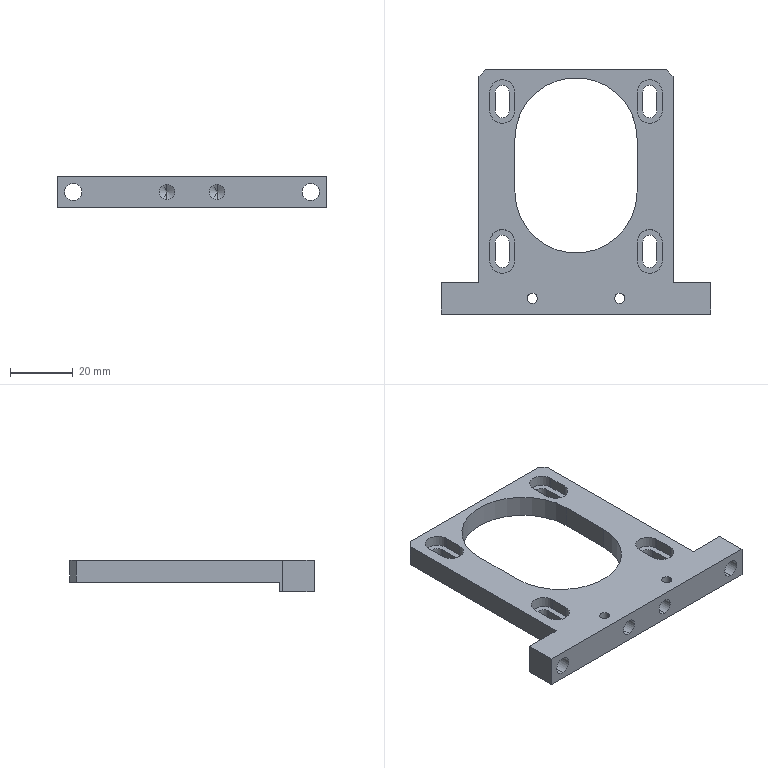Part | STEP file | 11-FG-SZ02111 | 1 solid | 70 faces | box 86 x 78 x 10 mm | volume 22329 mm3 | plane 36 | cylinder 30 | cone 4 | commonest cylinder face diameters 4.4 x8 8 x8 3.3 x4 5 x4 5.5 x4 39 x2